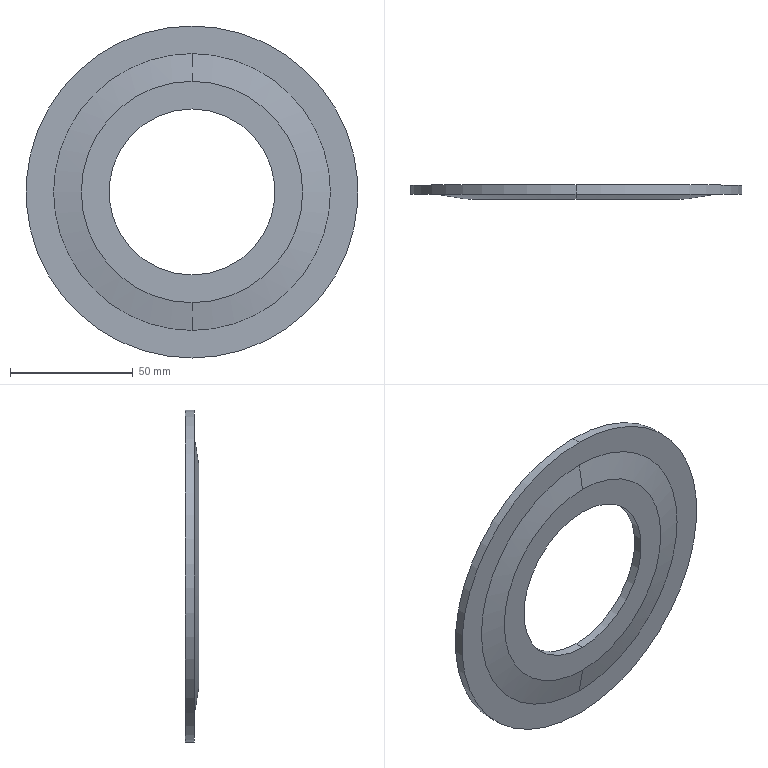Part | SolidWorks | features Revolution 1, Scale 1 | 1 solid | 12 faces | box 135 x 5.62 x 135 mm | volume 39683 mm3 | cone 4 | cylinder 4 | plane 4 | commonest cylinder face diameters 67.5 x2 135 x2
STEP:
#1=CARTESIAN_POINT('',(-18.,-1.373,45.));
#2=VERTEX_POINT('',#1);
#3=CARTESIAN_POINT('',(-18.,-1.373,-45.));
#4=VERTEX_POINT('',#3);
#5=CARTESIAN_POINT('',(-18.,-1.373,0.));
#6=DIRECTION('',(0.,1.,0.));
#7=DIRECTION('',(0.,0.,1.));
#8=AXIS2_PLACEMENT_3D('',#5,#6,#7);
#9=CIRCLE('',#8,45.);
#10=EDGE_CURVE('',#2,#4,#9,.T.);
#11=ORIENTED_EDGE('',*,*,#10,.T.);
#12=CARTESIAN_POINT('',(-18.,0.5023,-56.25));
#13=VERTEX_POINT('',#12);
#14=CARTESIAN_POINT('',(-18.,-1.373,-45.));
#15=DIRECTION('',(0.,0.1644,-0.9864));
#16=VECTOR('',#15,1000.);
#17=LINE('',#14,#16);
#18=EDGE_CURVE('',#4,#13,#17,.T.);
#19=ORIENTED_EDGE('',*,*,#18,.T.);
#20=CARTESIAN_POINT('',(-18.,0.5023,56.25));
#21=VERTEX_POINT('',#20);
#22=CARTESIAN_POINT('',(-18.,0.5023,0.));
#23=DIRECTION('',(0.,1.,0.));
#24=DIRECTION('',(0.,0.,1.));
#25=AXIS2_PLACEMENT_3D('',#22,#23,#24);
#26=CIRCLE('',#25,56.25);
#27=EDGE_CURVE('',#21,#13,#26,.T.);
#28=ORIENTED_EDGE('',*,*,#27,.F.);
#29=CARTESIAN_POINT('',(-18.,-1.373,45.));
#30=DIRECTION('',(0.,0.1644,0.9864));
#31=VECTOR('',#30,1000.);
#32=LINE('',#29,#31);
#33=EDGE_CURVE('',#2,#21,#32,.T.);
#34=ORIENTED_EDGE('',*,*,#33,.F.);
#35=EDGE_LOOP('',(#11,#19,#28,#34));
#36=FACE_OUTER_BOUND('',#35,.T.);
#37=CARTESIAN_POINT('',(-18.,-1.373,0.));
#38=DIRECTION('',(0.,1.,0.));
#39=DIRECTION('',(0.,0.,1.));
#40=AXIS2_PLACEMENT_3D('',#37,#38,#39);
#41=CONICAL_SURFACE('',#40,45.,1.406);
#42=ADVANCED_FACE('',(#36),#41,.T.);
#43=CARTESIAN_POINT('',(-18.,0.5023,67.5));
#44=VERTEX_POINT('',#43);
#45=CARTESIAN_POINT('',(-18.,0.5023,-67.5));
#46=VERTEX_POINT('',#45);
#47=CARTESIAN_POINT('',(-18.,0.5023,0.));
#48=DIRECTION('',(0.,1.,0.));
#49=DIRECTION('',(0.,0.,1.));
#50=AXIS2_PLACEMENT_3D('',#47,#48,#49);
#51=CIRCLE('',#50,67.5);
#52=EDGE_CURVE('',#44,#46,#51,.T.);
#53=ORIENTED_EDGE('',*,*,#52,.T.);
#54=CARTESIAN_POINT('',(-18.,4.247,-67.5));
#55=VERTEX_POINT('',#54);
#56=CARTESIAN_POINT('',(-18.,11.334,-67.5));
#57=DIRECTION('',(0.,1.,0.));
#58=VECTOR('',#57,1000.);
#59=LINE('',#56,#58);
#60=EDGE_CURVE('',#46,#55,#59,.T.);
#61=ORIENTED_EDGE('',*,*,#60,.T.);
#62=CARTESIAN_POINT('',(-18.,4.247,67.5));
#63=VERTEX_POINT('',#62);
#64=CARTESIAN_POINT('',(-18.,4.247,0.));
#65=DIRECTION('',(0.,1.,0.));
#66=DIRECTION('',(0.,0.,1.));
#67=AXIS2_PLACEMENT_3D('',#64,#65,#66);
#68=CIRCLE('',#67,67.5);
#69=EDGE_CURVE('',#63,#55,#68,.T.);
#70=ORIENTED_EDGE('',*,*,#69,.F.);
#71=CARTESIAN_POINT('',(-18.,11.334,67.5));
#72=DIRECTION('',(0.,1.,0.));
#73=VECTOR('',#72,1000.);
#74=LINE('',#71,#73);
#75=EDGE_CURVE('',#44,#63,#74,.T.);
#76=ORIENTED_EDGE('',*,*,#75,.F.);
#77=EDGE_LOOP('',(#53,#61,#70,#76));
#78=FACE_OUTER_BOUND('',#77,.T.);
#79=CARTESIAN_POINT('',(-18.,11.334,0.));
#80=DIRECTION('',(0.,1.,0.));
#81=DIRECTION('',(0.,0.,1.));
#82=AXIS2_PLACEMENT_3D('',#79,#80,#81);
#83=CYLINDRICAL_SURFACE('',#82,67.5);
#84=ADVANCED_FACE('',(#78),#83,.T.);
#85=CARTESIAN_POINT('',(-18.,2.377,-46.875));
#86=VERTEX_POINT('',#85);
#87=CARTESIAN_POINT('',(-18.,2.377,46.875));
#88=VERTEX_POINT('',#87);
#89=CARTESIAN_POINT('',(-18.,2.377,0.));
#90=DIRECTION('',(0.,1.,0.));
#91=DIRECTION('',(0.,0.,1.));
#92=AXIS2_PLACEMENT_3D('',#89,#90,#91);
#93=CIRCLE('',#92,46.875);
#94=EDGE_CURVE('',#86,#88,#93,.T.);
#95=ORIENTED_EDGE('',*,*,#94,.F.);
#96=CARTESIAN_POINT('',(-18.,4.247,-56.25));
#97=VERTEX_POINT('',#96);
#98=CARTESIAN_POINT('',(-18.,4.247,-56.25));
#99=DIRECTION('',(0.,0.1956,-0.9807));
#100=VECTOR('',#99,1000.);
#101=LINE('',#98,#100);
#102=EDGE_CURVE('',#86,#97,#101,.T.);
#103=ORIENTED_EDGE('',*,*,#102,.T.);
#104=CARTESIAN_POINT('',(-18.,4.247,56.25));
#105=VERTEX_POINT('',#104);
#106=CARTESIAN_POINT('',(-18.,4.247,0.));
#107=DIRECTION('',(0.,1.,0.));
#108=DIRECTION('',(0.,0.,1.));
#109=AXIS2_PLACEMENT_3D('',#106,#107,#108);
#110=CIRCLE('',#109,56.25);
#111=EDGE_CURVE('',#97,#105,#110,.T.);
#112=ORIENTED_EDGE('',*,*,#111,.T.);
#113=CARTESIAN_POINT('',(-18.,4.247,56.25));
#114=DIRECTION('',(0.,0.1956,0.9807));
#115=VECTOR('',#114,1000.);
#116=LINE('',#113,#115);
#117=EDGE_CURVE('',#88,#105,#116,.T.);
#118=ORIENTED_EDGE('',*,*,#117,.F.);
#119=EDGE_LOOP('',(#95,#103,#112,#118));
#120=FACE_OUTER_BOUND('',#119,.T.);
#121=CARTESIAN_POINT('',(-18.,4.247,0.));
#122=DIRECTION('',(0.,1.,0.));
#123=DIRECTION('',(0.,0.,1.));
#124=AXIS2_PLACEMENT_3D('',#121,#122,#123);
#125=CONICAL_SURFACE('',#124,56.25,1.374);
#126=ADVANCED_FACE('',(#120),#125,.F.);
#127=CARTESIAN_POINT('',(-18.,-1.373,-33.75));
#128=VERTEX_POINT('',#127);
#129=CARTESIAN_POINT('',(-18.,-1.373,33.75));
#130=VERTEX_POINT('',#129);
#131=CARTESIAN_POINT('',(-18.,-1.373,0.));
#132=DIRECTION('',(0.,1.,0.));
#133=DIRECTION('',(0.,0.,1.));
#134=AXIS2_PLACEMENT_3D('',#131,#132,#133);
#135=CIRCLE('',#134,33.75);
#136=EDGE_CURVE('',#128,#130,#135,.T.);
#137=ORIENTED_EDGE('',*,*,#136,.F.);
#138=CARTESIAN_POINT('',(-18.,2.377,-33.75));
#139=VERTEX_POINT('',#138);
#140=CARTESIAN_POINT('',(-18.,11.334,-33.75));
#141=DIRECTION('',(0.,1.,0.));
#142=VECTOR('',#141,1000.);
#143=LINE('',#140,#142);
#144=EDGE_CURVE('',#128,#139,#143,.T.);
#145=ORIENTED_EDGE('',*,*,#144,.T.);
#146=CARTESIAN_POINT('',(-18.,2.377,33.75));
#147=VERTEX_POINT('',#146);
#148=CARTESIAN_POINT('',(-18.,2.377,0.));
#149=DIRECTION('',(0.,1.,0.));
#150=DIRECTION('',(0.,0.,1.));
#151=AXIS2_PLACEMENT_3D('',#148,#149,#150);
#152=CIRCLE('',#151,33.75);
#153=EDGE_CURVE('',#139,#147,#152,.T.);
#154=ORIENTED_EDGE('',*,*,#153,.T.);
#155=CARTESIAN_POINT('',(-18.,11.334,33.75));
#156=DIRECTION('',(0.,1.,0.));
#157=VECTOR('',#156,1000.);
#158=LINE('',#155,#157);
#159=EDGE_CURVE('',#130,#147,#158,.T.);
#160=ORIENTED_EDGE('',*,*,#159,.F.);
#161=EDGE_LOOP('',(#137,#145,#154,#160));
#162=FACE_OUTER_BOUND('',#161,.T.);
#163=CARTESIAN_POINT('',(-18.,11.334,0.));
#164=DIRECTION('',(0.,1.,0.));
#165=DIRECTION('',(0.,0.,1.));
#166=AXIS2_PLACEMENT_3D('',#163,#164,#165);
#167=CYLINDRICAL_SURFACE('',#166,33.75);
#168=ADVANCED_FACE('',(#162),#167,.F.);
#169=ORIENTED_EDGE('',*,*,#10,.F.);
#170=CARTESIAN_POINT('',(-18.,-1.373,0.));
#171=DIRECTION('',(0.,1.,0.));
#172=DIRECTION('',(0.,0.,1.));
#173=AXIS2_PLACEMENT_3D('',#170,#171,#172);
#174=CIRCLE('',#173,45.);
#175=EDGE_CURVE('',#4,#2,#174,.T.);
#176=ORIENTED_EDGE('',*,*,#175,.F.);
#177=EDGE_LOOP('',(#169,#176));
#178=FACE_OUTER_BOUND('',#177,.T.);
#179=CARTESIAN_POINT('',(-18.,-1.373,0.));
#180=DIRECTION('',(0.,1.,0.));
#181=DIRECTION('',(0.,0.,1.));
#182=AXIS2_PLACEMENT_3D('',#179,#180,#181);
#183=CIRCLE('',#182,33.75);
#184=EDGE_CURVE('',#130,#128,#183,.T.);
#185=ORIENTED_EDGE('',*,*,#184,.T.);
#186=ORIENTED_EDGE('',*,*,#136,.T.);
#187=EDGE_LOOP('',(#185,#186));
#188=FACE_BOUND('',#187,.T.);
#189=CARTESIAN_POINT('',(15.75,-1.373,0.));
#190=DIRECTION('',(0.,1.,0.));
#191=DIRECTION('',(0.,0.,1.));
#192=AXIS2_PLACEMENT_3D('',#189,#190,#191);
#193=PLANE('',#192);
#194=ADVANCED_FACE('',(#178,#188),#193,.F.);
#195=ORIENTED_EDGE('',*,*,#144,.F.);
#196=ORIENTED_EDGE('',*,*,#184,.F.);
#197=ORIENTED_EDGE('',*,*,#159,.T.);
#198=CARTESIAN_POINT('',(-18.,2.377,0.));
#199=DIRECTION('',(0.,1.,0.));
#200=DIRECTION('',(0.,0.,1.));
#201=AXIS2_PLACEMENT_3D('',#198,#199,#200);
#202=CIRCLE('',#201,33.75);
#203=EDGE_CURVE('',#147,#139,#202,.T.);
#204=ORIENTED_EDGE('',*,*,#203,.T.);
#205=EDGE_LOOP('',(#195,#196,#197,#204));
#206=FACE_OUTER_BOUND('',#205,.T.);
#207=CARTESIAN_POINT('',(-18.,11.334,0.));
#208=DIRECTION('',(0.,1.,0.));
#209=DIRECTION('',(0.,0.,1.));
#210=AXIS2_PLACEMENT_3D('',#207,#208,#209);
#211=CYLINDRICAL_SURFACE('',#210,33.75);
#212=ADVANCED_FACE('',(#206),#211,.F.);
#213=ORIENTED_EDGE('',*,*,#203,.F.);
#214=ORIENTED_EDGE('',*,*,#153,.F.);
#215=EDGE_LOOP('',(#213,#214));
#216=FACE_BOUND('',#215,.T.);
#217=CARTESIAN_POINT('',(-18.,2.377,0.));
#218=DIRECTION('',(0.,1.,0.));
#219=DIRECTION('',(0.,0.,1.));
#220=AXIS2_PLACEMENT_3D('',#217,#218,#219);
#221=CIRCLE('',#220,46.875);
#222=EDGE_CURVE('',#88,#86,#221,.T.);
#223=ORIENTED_EDGE('',*,*,#222,.T.);
#224=ORIENTED_EDGE('',*,*,#94,.T.);
#225=EDGE_LOOP('',(#223,#224));
#226=FACE_OUTER_BOUND('',#225,.T.);
#227=CARTESIAN_POINT('',(15.75,2.377,0.));
#228=DIRECTION('',(0.,-1.,0.));
#229=DIRECTION('',(0.,0.,-1.));
#230=AXIS2_PLACEMENT_3D('',#227,#228,#229);
#231=PLANE('',#230);
#232=ADVANCED_FACE('',(#216,#226),#231,.F.);
#233=ORIENTED_EDGE('',*,*,#102,.F.);
#234=ORIENTED_EDGE('',*,*,#222,.F.);
#235=ORIENTED_EDGE('',*,*,#117,.T.);
#236=CARTESIAN_POINT('',(-18.,4.247,0.));
#237=DIRECTION('',(0.,1.,0.));
#238=DIRECTION('',(0.,0.,1.));
#239=AXIS2_PLACEMENT_3D('',#236,#237,#238);
#240=CIRCLE('',#239,56.25);
#241=EDGE_CURVE('',#105,#97,#240,.T.);
#242=ORIENTED_EDGE('',*,*,#241,.T.);
#243=EDGE_LOOP('',(#233,#234,#235,#242));
#244=FACE_OUTER_BOUND('',#243,.T.);
#245=CARTESIAN_POINT('',(-18.,4.247,0.));
#246=DIRECTION('',(0.,1.,0.));
#247=DIRECTION('',(0.,0.,1.));
#248=AXIS2_PLACEMENT_3D('',#245,#246,#247);
#249=CONICAL_SURFACE('',#248,56.25,1.374);
#250=ADVANCED_FACE('',(#244),#249,.F.);
#251=ORIENTED_EDGE('',*,*,#241,.F.);
#252=ORIENTED_EDGE('',*,*,#111,.F.);
#253=EDGE_LOOP('',(#251,#252));
#254=FACE_BOUND('',#253,.T.);
#255=ORIENTED_EDGE('',*,*,#69,.T.);
#256=CARTESIAN_POINT('',(-18.,4.247,0.));
#257=DIRECTION('',(0.,1.,0.));
#258=DIRECTION('',(0.,0.,1.));
#259=AXIS2_PLACEMENT_3D('',#256,#257,#258);
#260=CIRCLE('',#259,67.5);
#261=EDGE_CURVE('',#55,#63,#260,.T.);
#262=ORIENTED_EDGE('',*,*,#261,.T.);
#263=EDGE_LOOP('',(#255,#262));
#264=FACE_OUTER_BOUND('',#263,.T.);
#265=CARTESIAN_POINT('',(49.5,4.247,0.));
#266=DIRECTION('',(0.,-1.,0.));
#267=DIRECTION('',(0.,0.,-1.));
#268=AXIS2_PLACEMENT_3D('',#265,#266,#267);
#269=PLANE('',#268);
#270=ADVANCED_FACE('',(#254,#264),#269,.F.);
#271=ORIENTED_EDGE('',*,*,#60,.F.);
#272=CARTESIAN_POINT('',(-18.,0.5023,0.));
#273=DIRECTION('',(0.,1.,0.));
#274=DIRECTION('',(0.,0.,1.));
#275=AXIS2_PLACEMENT_3D('',#272,#273,#274);
#276=CIRCLE('',#275,67.5);
#277=EDGE_CURVE('',#46,#44,#276,.T.);
#278=ORIENTED_EDGE('',*,*,#277,.T.);
#279=ORIENTED_EDGE('',*,*,#75,.T.);
#280=ORIENTED_EDGE('',*,*,#261,.F.);
#281=EDGE_LOOP('',(#271,#278,#279,#280));
#282=FACE_OUTER_BOUND('',#281,.T.);
#283=CARTESIAN_POINT('',(-18.,11.334,0.));
#284=DIRECTION('',(0.,1.,0.));
#285=DIRECTION('',(0.,0.,1.));
#286=AXIS2_PLACEMENT_3D('',#283,#284,#285);
#287=CYLINDRICAL_SURFACE('',#286,67.5);
#288=ADVANCED_FACE('',(#282),#287,.T.);
#289=ORIENTED_EDGE('',*,*,#52,.F.);
#290=ORIENTED_EDGE('',*,*,#277,.F.);
#291=EDGE_LOOP('',(#289,#290));
#292=FACE_OUTER_BOUND('',#291,.T.);
#293=ORIENTED_EDGE('',*,*,#27,.T.);
#294=CARTESIAN_POINT('',(-18.,0.5023,0.));
#295=DIRECTION('',(0.,1.,0.));
#296=DIRECTION('',(0.,0.,1.));
#297=AXIS2_PLACEMENT_3D('',#294,#295,#296);
#298=CIRCLE('',#297,56.25);
#299=EDGE_CURVE('',#13,#21,#298,.T.);
#300=ORIENTED_EDGE('',*,*,#299,.T.);
#301=EDGE_LOOP('',(#293,#300));
#302=FACE_BOUND('',#301,.T.);
#303=CARTESIAN_POINT('',(49.5,0.5023,0.));
#304=DIRECTION('',(0.,1.,0.));
#305=DIRECTION('',(0.,0.,1.));
#306=AXIS2_PLACEMENT_3D('',#303,#304,#305);
#307=PLANE('',#306);
#308=ADVANCED_FACE('',(#292,#302),#307,.F.);
#309=ORIENTED_EDGE('',*,*,#18,.F.);
#310=ORIENTED_EDGE('',*,*,#175,.T.);
#311=ORIENTED_EDGE('',*,*,#33,.T.);
#312=ORIENTED_EDGE('',*,*,#299,.F.);
#313=EDGE_LOOP('',(#309,#310,#311,#312));
#314=FACE_OUTER_BOUND('',#313,.T.);
#315=CARTESIAN_POINT('',(-18.,-1.373,0.));
#316=DIRECTION('',(0.,1.,0.));
#317=DIRECTION('',(0.,0.,1.));
#318=AXIS2_PLACEMENT_3D('',#315,#316,#317);
#319=CONICAL_SURFACE('',#318,45.,1.406);
#320=ADVANCED_FACE('',(#314),#319,.T.);
#321=CLOSED_SHELL('',(#42,#84,#126,#168,#194,#212,#232,#250,#270,#288,#308,#320));
#322=MANIFOLD_SOLID_BREP('',#321);
#323=CARTESIAN_POINT('',(0.,0.,0.));
#324=DIRECTION('',(0.,0.,1.));
#325=DIRECTION('',(1.,0.,0.));
#326=AXIS2_PLACEMENT_3D('',#323,#324,#325);
#327=(LENGTH_UNIT()NAMED_UNIT(*)SI_UNIT(.MILLI.,.METRE.));
#328=UNCERTAINTY_MEASURE_WITH_UNIT(LENGTH_MEASURE(0.00001),#327,'','');
#329=(NAMED_UNIT(*)PLANE_ANGLE_UNIT()SI_UNIT($,.RADIAN.));
#330=(NAMED_UNIT(*)SI_UNIT($,.STERADIAN.)SOLID_ANGLE_UNIT());
#331=(GEOMETRIC_REPRESENTATION_CONTEXT(3)GLOBAL_UNCERTAINTY_ASSIGNED_CONTEXT((#328))GLOBAL_UNIT_ASSIGNED_CONTEXT((#327,#329,#330))REPRESENTATION_CONTEXT('',''));
#332=ADVANCED_BREP_SHAPE_REPRESENTATION('',(#322,#326),#331);